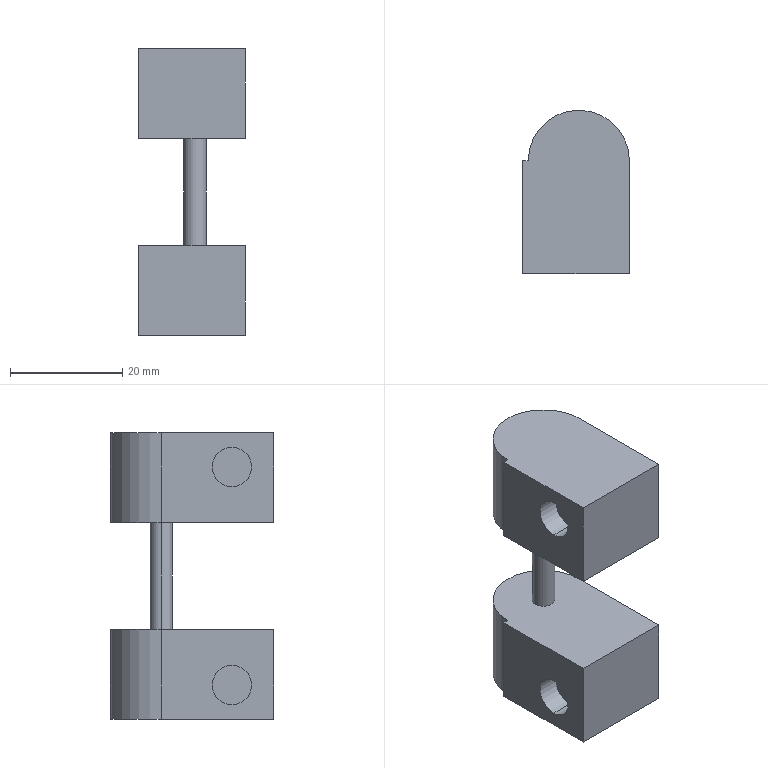Part | STEP file | Hinge side | 1 solid | 22 faces | box 19 x 29 x 51 mm | volume 16162 mm3 | plane 14 | cylinder 8 | commonest cylinder face diameters 7 x4 4 x2 18 x2
STEP:
#1=CARTESIAN_POINT('',(0.,0.,0.));
#2=DIRECTION('',(0.,0.,1.));
#3=DIRECTION('',(1.,0.,0.));
#4=AXIS2_PLACEMENT_3D('',#1,#2,#3);
#5=CARTESIAN_POINT('',(-6.,7.4,5.4));
#6=VERTEX_POINT('',#5);
#7=CARTESIAN_POINT('',(-10.,7.4,5.4));
#8=VERTEX_POINT('',#7);
#9=CARTESIAN_POINT('',(-6.,7.4,5.4));
#10=DIRECTION('',(-1.,0.,0.));
#11=VECTOR('',#10,1.);
#12=LINE('',#9,#11);
#13=CARTESIAN_POINT('',(-6.,7.4,1.9));
#14=DIRECTION('',(-1.,0.,0.));
#15=DIRECTION('',(0.,0.,1.));
#16=AXIS2_PLACEMENT_3D('',#13,#14,#15);
#17=CYLINDRICAL_SURFACE('',#16,3.5);
#18=CARTESIAN_POINT('',(6.283,0.));
#19=DIRECTION('',(0.,1.));
#20=VECTOR('',#19,1.);
#21=LINE('',#18,#20);
#22=(GEOMETRIC_REPRESENTATION_CONTEXT(2)PARAMETRIC_REPRESENTATION_CONTEXT()REPRESENTATION_CONTEXT('',''));
#23=DEFINITIONAL_REPRESENTATION('',(#21),#22);
#24=PCURVE('',#17,#23);
#25=CARTESIAN_POINT('',(-6.,7.4,1.9));
#26=DIRECTION('',(-1.,0.,0.));
#27=DIRECTION('',(0.,0.,1.));
#28=AXIS2_PLACEMENT_3D('',#25,#26,#27);
#29=CYLINDRICAL_SURFACE('',#28,3.5);
#30=CARTESIAN_POINT('',(0.,0.));
#31=DIRECTION('',(0.,1.));
#32=VECTOR('',#31,1.);
#33=LINE('',#30,#32);
#34=(GEOMETRIC_REPRESENTATION_CONTEXT(2)PARAMETRIC_REPRESENTATION_CONTEXT()REPRESENTATION_CONTEXT('',''));
#35=DEFINITIONAL_REPRESENTATION('',(#33),#34);
#36=PCURVE('',#29,#35);
#37=SURFACE_CURVE('',#12,(#24,#36),.PCURVE_S1.);
#38=EDGE_CURVE('',#6,#8,#37,.T.);
#39=ORIENTED_EDGE('',*,*,#38,.T.);
#40=CARTESIAN_POINT('',(-10.,7.4,-1.6));
#41=VERTEX_POINT('',#40);
#42=CARTESIAN_POINT('',(-10.,7.4,1.9));
#43=DIRECTION('',(-1.,0.,0.));
#44=DIRECTION('',(0.,0.,-1.));
#45=AXIS2_PLACEMENT_3D('',#42,#43,#44);
#46=CIRCLE('',#45,3.5);
#47=CARTESIAN_POINT('',(3.142,4.));
#48=DIRECTION('',(1.,0.));
#49=VECTOR('',#48,1.);
#50=LINE('',#47,#49);
#51=(GEOMETRIC_REPRESENTATION_CONTEXT(2)PARAMETRIC_REPRESENTATION_CONTEXT()REPRESENTATION_CONTEXT('',''));
#52=DEFINITIONAL_REPRESENTATION('',(#50),#51);
#53=PCURVE('',#17,#52);
#54=CARTESIAN_POINT('',(-10.,20.,8.));
#55=DIRECTION('',(-1.,0.,0.));
#56=DIRECTION('',(0.,0.,1.));
#57=AXIS2_PLACEMENT_3D('',#54,#55,#56);
#58=PLANE('',#57);
#59=CARTESIAN_POINT('',(-6.1,-12.6));
#60=DIRECTION('',(-1.,0.));
#61=AXIS2_PLACEMENT_2D('',#59,#60);
#62=CIRCLE('',#61,3.5);
#63=(GEOMETRIC_REPRESENTATION_CONTEXT(2)PARAMETRIC_REPRESENTATION_CONTEXT()REPRESENTATION_CONTEXT('',''));
#64=DEFINITIONAL_REPRESENTATION('',(#62),#63);
#65=PCURVE('',#58,#64);
#66=SURFACE_CURVE('',#46,(#53,#65),.PCURVE_S1.);
#67=EDGE_CURVE('',#41,#8,#66,.T.);
#68=ORIENTED_EDGE('',*,*,#67,.F.);
#69=CARTESIAN_POINT('',(-6.,7.4,-1.6));
#70=VERTEX_POINT('',#69);
#71=CARTESIAN_POINT('',(-6.,7.4,-1.6));
#72=DIRECTION('',(-1.,0.,0.));
#73=VECTOR('',#72,1.);
#74=LINE('',#71,#73);
#75=CARTESIAN_POINT('',(3.142,0.));
#76=DIRECTION('',(0.,1.));
#77=VECTOR('',#76,1.);
#78=LINE('',#75,#77);
#79=(GEOMETRIC_REPRESENTATION_CONTEXT(2)PARAMETRIC_REPRESENTATION_CONTEXT()REPRESENTATION_CONTEXT('',''));
#80=DEFINITIONAL_REPRESENTATION('',(#78),#79);
#81=PCURVE('',#17,#80);
#82=CARTESIAN_POINT('',(3.142,0.));
#83=DIRECTION('',(0.,1.));
#84=VECTOR('',#83,1.);
#85=LINE('',#82,#84);
#86=(GEOMETRIC_REPRESENTATION_CONTEXT(2)PARAMETRIC_REPRESENTATION_CONTEXT()REPRESENTATION_CONTEXT('',''));
#87=DEFINITIONAL_REPRESENTATION('',(#85),#86);
#88=PCURVE('',#29,#87);
#89=SURFACE_CURVE('',#74,(#81,#88),.PCURVE_S1.);
#90=EDGE_CURVE('',#70,#41,#89,.T.);
#91=ORIENTED_EDGE('',*,*,#90,.F.);
#92=CARTESIAN_POINT('',(-6.,7.4,1.9));
#93=DIRECTION('',(-1.,0.,0.));
#94=DIRECTION('',(0.,0.,-1.));
#95=AXIS2_PLACEMENT_3D('',#92,#93,#94);
#96=CIRCLE('',#95,3.5);
#97=CARTESIAN_POINT('',(3.142,0.));
#98=DIRECTION('',(1.,0.));
#99=VECTOR('',#98,1.);
#100=LINE('',#97,#99);
#101=(GEOMETRIC_REPRESENTATION_CONTEXT(2)PARAMETRIC_REPRESENTATION_CONTEXT()REPRESENTATION_CONTEXT('',''));
#102=DEFINITIONAL_REPRESENTATION('',(#100),#101);
#103=PCURVE('',#17,#102);
#104=CARTESIAN_POINT('',(-6.,7.4,1.9));
#105=DIRECTION('',(1.,0.,0.));
#106=DIRECTION('',(0.,0.,-1.));
#107=AXIS2_PLACEMENT_3D('',#104,#105,#106);
#108=PLANE('',#107);
#109=CARTESIAN_POINT('',(3.5,0.));
#110=CARTESIAN_POINT('',(3.5,-6.062));
#111=CARTESIAN_POINT('',(-1.75,-3.031));
#112=CARTESIAN_POINT('',(-7.,0.));
#113=CARTESIAN_POINT('',(-1.75,3.031));
#114=CARTESIAN_POINT('',(3.5,6.062));
#115=CARTESIAN_POINT('',(3.5,0.));
#116=(BOUNDED_CURVE()B_SPLINE_CURVE(2,(#109,#110,#111,#112,#113,#114,#115),.UNSPECIFIED.,.T.,.F.)B_SPLINE_CURVE_WITH_KNOTS((1,2,2,2,2,1),(-2.094,0.,2.094,4.189,6.283,8.378),.UNSPECIFIED.)CURVE()GEOMETRIC_REPRESENTATION_ITEM()RATIONAL_B_SPLINE_CURVE((1.,0.5,1.,0.5,1.,0.5,1.))REPRESENTATION_ITEM(''));
#117=(GEOMETRIC_REPRESENTATION_CONTEXT(2)PARAMETRIC_REPRESENTATION_CONTEXT()REPRESENTATION_CONTEXT('',''));
#118=DEFINITIONAL_REPRESENTATION('',(#116),#117);
#119=PCURVE('',#108,#118);
#120=SURFACE_CURVE('',#96,(#103,#119),.PCURVE_S1.);
#121=EDGE_CURVE('',#70,#6,#120,.T.);
#122=ORIENTED_EDGE('',*,*,#121,.T.);
#123=EDGE_LOOP('',(#39,#68,#91,#122));
#124=FACE_BOUND('',#123,.F.);
#125=ADVANCED_FACE('',(#124),#17,.F.);
#126=CARTESIAN_POINT('',(-6.,7.4,-33.4));
#127=VERTEX_POINT('',#126);
#128=CARTESIAN_POINT('',(-10.,7.4,-33.4));
#129=VERTEX_POINT('',#128);
#130=CARTESIAN_POINT('',(-6.,7.4,-33.4));
#131=DIRECTION('',(-1.,0.,0.));
#132=VECTOR('',#131,1.);
#133=LINE('',#130,#132);
#134=CARTESIAN_POINT('',(-6.,7.4,-36.9));
#135=DIRECTION('',(-1.,0.,0.));
#136=DIRECTION('',(0.,0.,1.));
#137=AXIS2_PLACEMENT_3D('',#134,#135,#136);
#138=CYLINDRICAL_SURFACE('',#137,3.5);
#139=CARTESIAN_POINT('',(6.283,0.));
#140=DIRECTION('',(0.,1.));
#141=VECTOR('',#140,1.);
#142=LINE('',#139,#141);
#143=(GEOMETRIC_REPRESENTATION_CONTEXT(2)PARAMETRIC_REPRESENTATION_CONTEXT()REPRESENTATION_CONTEXT('',''));
#144=DEFINITIONAL_REPRESENTATION('',(#142),#143);
#145=PCURVE('',#138,#144);
#146=CARTESIAN_POINT('',(-6.,7.4,-36.9));
#147=DIRECTION('',(-1.,0.,0.));
#148=DIRECTION('',(0.,0.,1.));
#149=AXIS2_PLACEMENT_3D('',#146,#147,#148);
#150=CYLINDRICAL_SURFACE('',#149,3.5);
#151=CARTESIAN_POINT('',(0.,0.));
#152=DIRECTION('',(0.,1.));
#153=VECTOR('',#152,1.);
#154=LINE('',#151,#153);
#155=(GEOMETRIC_REPRESENTATION_CONTEXT(2)PARAMETRIC_REPRESENTATION_CONTEXT()REPRESENTATION_CONTEXT('',''));
#156=DEFINITIONAL_REPRESENTATION('',(#154),#155);
#157=PCURVE('',#150,#156);
#158=SURFACE_CURVE('',#133,(#145,#157),.PCURVE_S1.);
#159=EDGE_CURVE('',#127,#129,#158,.T.);
#160=ORIENTED_EDGE('',*,*,#159,.T.);
#161=CARTESIAN_POINT('',(-10.,7.4,-40.4));
#162=VERTEX_POINT('',#161);
#163=CARTESIAN_POINT('',(-10.,7.4,-36.9));
#164=DIRECTION('',(-1.,0.,0.));
#165=DIRECTION('',(0.,0.,1.));
#166=AXIS2_PLACEMENT_3D('',#163,#164,#165);
#167=CIRCLE('',#166,3.5);
#168=CARTESIAN_POINT('',(0.,4.));
#169=DIRECTION('',(1.,0.));
#170=VECTOR('',#169,1.);
#171=LINE('',#168,#170);
#172=(GEOMETRIC_REPRESENTATION_CONTEXT(2)PARAMETRIC_REPRESENTATION_CONTEXT()REPRESENTATION_CONTEXT('',''));
#173=DEFINITIONAL_REPRESENTATION('',(#171),#172);
#174=PCURVE('',#138,#173);
#175=CARTESIAN_POINT('',(-10.,20.,-43.));
#176=DIRECTION('',(1.,0.,0.));
#177=DIRECTION('',(0.,0.,-1.));
#178=AXIS2_PLACEMENT_3D('',#175,#176,#177);
#179=PLANE('',#178);
#180=CARTESIAN_POINT('',(-9.6,-12.6));
#181=CARTESIAN_POINT('',(-9.6,-6.538));
#182=CARTESIAN_POINT('',(-4.35,-9.569));
#183=CARTESIAN_POINT('',(0.9,-12.6));
#184=CARTESIAN_POINT('',(-4.35,-15.631));
#185=CARTESIAN_POINT('',(-9.6,-18.662));
#186=CARTESIAN_POINT('',(-9.6,-12.6));
#187=(BOUNDED_CURVE()B_SPLINE_CURVE(2,(#180,#181,#182,#183,#184,#185,#186),.UNSPECIFIED.,.T.,.F.)B_SPLINE_CURVE_WITH_KNOTS((1,2,2,2,2,1),(-2.094,0.,2.094,4.189,6.283,8.378),.UNSPECIFIED.)CURVE()GEOMETRIC_REPRESENTATION_ITEM()RATIONAL_B_SPLINE_CURVE((1.,0.5,1.,0.5,1.,0.5,1.))REPRESENTATION_ITEM(''));
#188=(GEOMETRIC_REPRESENTATION_CONTEXT(2)PARAMETRIC_REPRESENTATION_CONTEXT()REPRESENTATION_CONTEXT('',''));
#189=DEFINITIONAL_REPRESENTATION('',(#187),#188);
#190=PCURVE('',#179,#189);
#191=SURFACE_CURVE('',#167,(#174,#190),.PCURVE_S1.);
#192=EDGE_CURVE('',#162,#129,#191,.T.);
#193=ORIENTED_EDGE('',*,*,#192,.F.);
#194=CARTESIAN_POINT('',(-6.,7.4,-40.4));
#195=VERTEX_POINT('',#194);
#196=CARTESIAN_POINT('',(-6.,7.4,-40.4));
#197=DIRECTION('',(-1.,0.,0.));
#198=VECTOR('',#197,1.);
#199=LINE('',#196,#198);
#200=CARTESIAN_POINT('',(3.142,0.));
#201=DIRECTION('',(0.,1.));
#202=VECTOR('',#201,1.);
#203=LINE('',#200,#202);
#204=(GEOMETRIC_REPRESENTATION_CONTEXT(2)PARAMETRIC_REPRESENTATION_CONTEXT()REPRESENTATION_CONTEXT('',''));
#205=DEFINITIONAL_REPRESENTATION('',(#203),#204);
#206=PCURVE('',#138,#205);
#207=CARTESIAN_POINT('',(3.142,0.));
#208=DIRECTION('',(0.,1.));
#209=VECTOR('',#208,1.);
#210=LINE('',#207,#209);
#211=(GEOMETRIC_REPRESENTATION_CONTEXT(2)PARAMETRIC_REPRESENTATION_CONTEXT()REPRESENTATION_CONTEXT('',''));
#212=DEFINITIONAL_REPRESENTATION('',(#210),#211);
#213=PCURVE('',#150,#212);
#214=SURFACE_CURVE('',#199,(#206,#213),.PCURVE_S1.);
#215=EDGE_CURVE('',#195,#162,#214,.T.);
#216=ORIENTED_EDGE('',*,*,#215,.F.);
#217=CARTESIAN_POINT('',(-6.,7.4,-36.9));
#218=DIRECTION('',(-1.,0.,0.));
#219=DIRECTION('',(0.,0.,1.));
#220=AXIS2_PLACEMENT_3D('',#217,#218,#219);
#221=CIRCLE('',#220,3.5);
#222=CARTESIAN_POINT('',(0.,0.));
#223=DIRECTION('',(1.,0.));
#224=VECTOR('',#223,1.);
#225=LINE('',#222,#224);
#226=(GEOMETRIC_REPRESENTATION_CONTEXT(2)PARAMETRIC_REPRESENTATION_CONTEXT()REPRESENTATION_CONTEXT('',''));
#227=DEFINITIONAL_REPRESENTATION('',(#225),#226);
#228=PCURVE('',#138,#227);
#229=CARTESIAN_POINT('',(-6.,7.4,-36.9));
#230=DIRECTION('',(-1.,0.,0.));
#231=DIRECTION('',(0.,0.,1.));
#232=AXIS2_PLACEMENT_3D('',#229,#230,#231);
#233=PLANE('',#232);
#234=CARTESIAN_POINT('',(0.,0.));
#235=DIRECTION('',(1.,0.));
#236=AXIS2_PLACEMENT_2D('',#234,#235);
#237=CIRCLE('',#236,3.5);
#238=(GEOMETRIC_REPRESENTATION_CONTEXT(2)PARAMETRIC_REPRESENTATION_CONTEXT()REPRESENTATION_CONTEXT('',''));
#239=DEFINITIONAL_REPRESENTATION('',(#237),#238);
#240=PCURVE('',#233,#239);
#241=SURFACE_CURVE('',#221,(#228,#240),.PCURVE_S1.);
#242=EDGE_CURVE('',#195,#127,#241,.T.);
#243=ORIENTED_EDGE('',*,*,#242,.T.);
#244=EDGE_LOOP('',(#160,#193,#216,#243));
#245=FACE_BOUND('',#244,.F.);
#246=ADVANCED_FACE('',(#245),#138,.F.);
#247=CARTESIAN_POINT('',(-2.,20.,-27.));
#248=VERTEX_POINT('',#247);
#249=CARTESIAN_POINT('',(2.,20.,-27.));
#250=VERTEX_POINT('',#249);
#251=CARTESIAN_POINT('',(0.,20.,-27.));
#252=DIRECTION('',(0.,0.,-1.));
#253=DIRECTION('',(-1.,0.,0.));
#254=AXIS2_PLACEMENT_3D('',#251,#252,#253);
#255=CIRCLE('',#254,2.);
#256=CARTESIAN_POINT('',(0.,20.,-27.));
#257=DIRECTION('',(0.,0.,1.));
#258=DIRECTION('',(1.,0.,0.));
#259=AXIS2_PLACEMENT_3D('',#256,#257,#258);
#260=CYLINDRICAL_SURFACE('',#259,2.);
#261=CARTESIAN_POINT('',(3.142,0.));
#262=DIRECTION('',(-1.,0.));
#263=VECTOR('',#262,1.);
#264=LINE('',#261,#263);
#265=(GEOMETRIC_REPRESENTATION_CONTEXT(2)PARAMETRIC_REPRESENTATION_CONTEXT()REPRESENTATION_CONTEXT('',''));
#266=DEFINITIONAL_REPRESENTATION('',(#264),#265);
#267=PCURVE('',#260,#266);
#268=CARTESIAN_POINT('',(-9.,20.,-27.));
#269=DIRECTION('',(0.,0.,1.));
#270=DIRECTION('',(1.,0.,0.));
#271=AXIS2_PLACEMENT_3D('',#268,#269,#270);
#272=PLANE('',#271);
#273=CARTESIAN_POINT('',(7.,0.));
#274=CARTESIAN_POINT('',(7.,3.464));
#275=CARTESIAN_POINT('',(10.,1.732));
#276=CARTESIAN_POINT('',(13.,0.));
#277=CARTESIAN_POINT('',(10.,-1.732));
#278=CARTESIAN_POINT('',(7.,-3.464));
#279=CARTESIAN_POINT('',(7.,0.));
#280=(BOUNDED_CURVE()B_SPLINE_CURVE(2,(#273,#274,#275,#276,#277,#278,#279),.UNSPECIFIED.,.T.,.F.)B_SPLINE_CURVE_WITH_KNOTS((1,2,2,2,2,1),(-2.094,0.,2.094,4.189,6.283,8.378),.UNSPECIFIED.)CURVE()GEOMETRIC_REPRESENTATION_ITEM()RATIONAL_B_SPLINE_CURVE((1.,0.5,1.,0.5,1.,0.5,1.))REPRESENTATION_ITEM(''));
#281=(GEOMETRIC_REPRESENTATION_CONTEXT(2)PARAMETRIC_REPRESENTATION_CONTEXT()REPRESENTATION_CONTEXT('',''));
#282=DEFINITIONAL_REPRESENTATION('',(#280),#281);
#283=PCURVE('',#272,#282);
#284=SURFACE_CURVE('',#255,(#267,#283),.PCURVE_S1.);
#285=EDGE_CURVE('',#248,#250,#284,.T.);
#286=ORIENTED_EDGE('',*,*,#285,.F.);
#287=CARTESIAN_POINT('',(-2.,20.,-8.));
#288=VERTEX_POINT('',#287);
#289=CARTESIAN_POINT('',(-2.,20.,-27.));
#290=DIRECTION('',(0.,0.,1.));
#291=VECTOR('',#290,1.);
#292=LINE('',#289,#291);
#293=CARTESIAN_POINT('',(3.142,0.));
#294=DIRECTION('',(0.,1.));
#295=VECTOR('',#294,1.);
#296=LINE('',#293,#295);
#297=(GEOMETRIC_REPRESENTATION_CONTEXT(2)PARAMETRIC_REPRESENTATION_CONTEXT()REPRESENTATION_CONTEXT('',''));
#298=DEFINITIONAL_REPRESENTATION('',(#296),#297);
#299=PCURVE('',#260,#298);
#300=CARTESIAN_POINT('',(0.,20.,-27.));
#301=DIRECTION('',(0.,0.,1.));
#302=DIRECTION('',(1.,0.,0.));
#303=AXIS2_PLACEMENT_3D('',#300,#301,#302);
#304=CYLINDRICAL_SURFACE('',#303,2.);
#305=CARTESIAN_POINT('',(3.142,0.));
#306=DIRECTION('',(0.,1.));
#307=VECTOR('',#306,1.);
#308=LINE('',#305,#307);
#309=(GEOMETRIC_REPRESENTATION_CONTEXT(2)PARAMETRIC_REPRESENTATION_CONTEXT()REPRESENTATION_CONTEXT('',''));
#310=DEFINITIONAL_REPRESENTATION('',(#308),#309);
#311=PCURVE('',#304,#310);
#312=SURFACE_CURVE('',#292,(#299,#311),.PCURVE_S1.);
#313=EDGE_CURVE('',#248,#288,#312,.T.);
#314=ORIENTED_EDGE('',*,*,#313,.T.);
#315=CARTESIAN_POINT('',(2.,20.,-8.));
#316=VERTEX_POINT('',#315);
#317=CARTESIAN_POINT('',(0.,20.,-8.));
#318=DIRECTION('',(0.,0.,-1.));
#319=DIRECTION('',(1.,0.,0.));
#320=AXIS2_PLACEMENT_3D('',#317,#318,#319);
#321=CIRCLE('',#320,2.);
#322=CARTESIAN_POINT('',(6.283,19.));
#323=DIRECTION('',(-1.,0.));
#324=VECTOR('',#323,1.);
#325=LINE('',#322,#324);
#326=(GEOMETRIC_REPRESENTATION_CONTEXT(2)PARAMETRIC_REPRESENTATION_CONTEXT()REPRESENTATION_CONTEXT('',''));
#327=DEFINITIONAL_REPRESENTATION('',(#325),#326);
#328=PCURVE('',#260,#327);
#329=CARTESIAN_POINT('',(-9.,20.,-8.));
#330=DIRECTION('',(0.,0.,1.));
#331=DIRECTION('',(1.,0.,0.));
#332=AXIS2_PLACEMENT_3D('',#329,#330,#331);
#333=PLANE('',#332);
#334=CARTESIAN_POINT('',(11.,0.));
#335=CARTESIAN_POINT('',(11.,-3.464));
#336=CARTESIAN_POINT('',(8.,-1.732));
#337=CARTESIAN_POINT('',(5.,0.));
#338=CARTESIAN_POINT('',(8.,1.732));
#339=CARTESIAN_POINT('',(11.,3.464));
#340=CARTESIAN_POINT('',(11.,0.));
#341=(BOUNDED_CURVE()B_SPLINE_CURVE(2,(#334,#335,#336,#337,#338,#339,#340),.UNSPECIFIED.,.T.,.F.)B_SPLINE_CURVE_WITH_KNOTS((1,2,2,2,2,1),(-2.094,0.,2.094,4.189,6.283,8.378),.UNSPECIFIED.)CURVE()GEOMETRIC_REPRESENTATION_ITEM()RATIONAL_B_SPLINE_CURVE((1.,0.5,1.,0.5,1.,0.5,1.))REPRESENTATION_ITEM(''));
#342=(GEOMETRIC_REPRESENTATION_CONTEXT(2)PARAMETRIC_REPRESENTATION_CONTEXT()REPRESENTATION_CONTEXT('',''));
#343=DEFINITIONAL_REPRESENTATION('',(#341),#342);
#344=PCURVE('',#333,#343);
#345=SURFACE_CURVE('',#321,(#328,#344),.PCURVE_S1.);
#346=EDGE_CURVE('',#288,#316,#345,.T.);
#347=ORIENTED_EDGE('',*,*,#346,.T.);
#348=CARTESIAN_POINT('',(2.,20.,-27.));
#349=DIRECTION('',(0.,0.,1.));
#350=VECTOR('',#349,1.);
#351=LINE('',#348,#350);
#352=CARTESIAN_POINT('',(0.,0.));
#353=DIRECTION('',(0.,1.));
#354=VECTOR('',#353,1.);
#355=LINE('',#352,#354);
#356=(GEOMETRIC_REPRESENTATION_CONTEXT(2)PARAMETRIC_REPRESENTATION_CONTEXT()REPRESENTATION_CONTEXT('',''));
#357=DEFINITIONAL_REPRESENTATION('',(#355),#356);
#358=PCURVE('',#260,#357);
#359=CARTESIAN_POINT('',(6.283,0.));
#360=DIRECTION('',(0.,1.));
#361=VECTOR('',#360,1.);
#362=LINE('',#359,#361);
#363=(GEOMETRIC_REPRESENTATION_CONTEXT(2)PARAMETRIC_REPRESENTATION_CONTEXT()REPRESENTATION_CONTEXT('',''));
#364=DEFINITIONAL_REPRESENTATION('',(#362),#363);
#365=PCURVE('',#304,#364);
#366=SURFACE_CURVE('',#351,(#358,#365),.PCURVE_S1.);
#367=EDGE_CURVE('',#250,#316,#366,.T.);
#368=ORIENTED_EDGE('',*,*,#367,.F.);
#369=EDGE_LOOP('',(#286,#314,#347,#368));
#370=FACE_BOUND('',#369,.T.);
#371=ADVANCED_FACE('',(#370),#260,.T.);
#372=CARTESIAN_POINT('',(9.,0.,8.));
#373=VERTEX_POINT('',#372);
#374=CARTESIAN_POINT('',(9.,0.,-8.));
#375=VERTEX_POINT('',#374);
#376=CARTESIAN_POINT('',(9.,0.,-8.));
#377=DIRECTION('',(0.,0.,-1.));
#378=VECTOR('',#377,1.);
#379=LINE('',#376,#378);
#380=CARTESIAN_POINT('',(9.,20.,-8.));
#381=DIRECTION('',(-1.,0.,0.));
#382=DIRECTION('',(0.,0.,1.));
#383=AXIS2_PLACEMENT_3D('',#380,#381,#382);
#384=PLANE('',#383);
#385=CARTESIAN_POINT('',(0.,-20.));
#386=DIRECTION('',(-1.,0.));
#387=VECTOR('',#386,1.);
#388=LINE('',#385,#387);
#389=(GEOMETRIC_REPRESENTATION_CONTEXT(2)PARAMETRIC_REPRESENTATION_CONTEXT()REPRESENTATION_CONTEXT('',''));
#390=DEFINITIONAL_REPRESENTATION('',(#388),#389);
#391=PCURVE('',#384,#390);
#392=CARTESIAN_POINT('',(0.,0.,0.));
#393=DIRECTION('',(0.,1.,0.));
#394=DIRECTION('',(0.,0.,1.));
#395=AXIS2_PLACEMENT_3D('',#392,#393,#394);
#396=PLANE('',#395);
#397=CARTESIAN_POINT('',(-8.,9.));
#398=DIRECTION('',(-1.,0.));
#399=VECTOR('',#398,1.);
#400=LINE('',#397,#399);
#401=(GEOMETRIC_REPRESENTATION_CONTEXT(2)PARAMETRIC_REPRESENTATION_CONTEXT()REPRESENTATION_CONTEXT('',''));
#402=DEFINITIONAL_REPRESENTATION('',(#400),#401);
#403=PCURVE('',#396,#402);
#404=SURFACE_CURVE('',#379,(#391,#403),.PCURVE_S1.);
#405=EDGE_CURVE('',#373,#375,#404,.T.);
#406=ORIENTED_EDGE('',*,*,#405,.T.);
#407=CARTESIAN_POINT('',(9.,20.,-8.));
#408=VERTEX_POINT('',#407);
#409=CARTESIAN_POINT('',(9.,20.,-8.));
#410=DIRECTION('',(0.,-1.,0.));
#411=VECTOR('',#410,1.);
#412=LINE('',#409,#411);
#413=CARTESIAN_POINT('',(0.,0.));
#414=DIRECTION('',(0.,-1.));
#415=VECTOR('',#414,1.);
#416=LINE('',#413,#415);
#417=(GEOMETRIC_REPRESENTATION_CONTEXT(2)PARAMETRIC_REPRESENTATION_CONTEXT()REPRESENTATION_CONTEXT('',''));
#418=DEFINITIONAL_REPRESENTATION('',(#416),#417);
#419=PCURVE('',#384,#418);
#420=CARTESIAN_POINT('',(18.,0.));
#421=DIRECTION('',(0.,-1.));
#422=VECTOR('',#421,1.);
#423=LINE('',#420,#422);
#424=(GEOMETRIC_REPRESENTATION_CONTEXT(2)PARAMETRIC_REPRESENTATION_CONTEXT()REPRESENTATION_CONTEXT('',''));
#425=DEFINITIONAL_REPRESENTATION('',(#423),#424);
#426=PCURVE('',#333,#425);
#427=SURFACE_CURVE('',#412,(#419,#426),.PCURVE_S1.);
#428=EDGE_CURVE('',#408,#375,#427,.T.);
#429=ORIENTED_EDGE('',*,*,#428,.F.);
#430=CARTESIAN_POINT('',(9.,20.,8.));
#431=VERTEX_POINT('',#430);
#432=CARTESIAN_POINT('',(9.,20.,-8.));
#433=DIRECTION('',(0.,0.,-1.));
#434=VECTOR('',#433,1.);
#435=LINE('',#432,#434);
#436=CARTESIAN_POINT('',(0.,0.));
#437=DIRECTION('',(-1.,0.));
#438=VECTOR('',#437,1.);
#439=LINE('',#436,#438);
#440=(GEOMETRIC_REPRESENTATION_CONTEXT(2)PARAMETRIC_REPRESENTATION_CONTEXT()REPRESENTATION_CONTEXT('',''));
#441=DEFINITIONAL_REPRESENTATION('',(#439),#440);
#442=PCURVE('',#384,#441);
#443=CARTESIAN_POINT('',(0.,20.,8.));
#444=DIRECTION('',(0.,0.,-1.));
#445=DIRECTION('',(-1.,0.,0.));
#446=AXIS2_PLACEMENT_3D('',#443,#444,#445);
#447=CYLINDRICAL_SURFACE('',#446,9.);
#448=CARTESIAN_POINT('',(3.142,16.));
#449=DIRECTION('',(0.,1.));
#450=VECTOR('',#449,1.);
#451=LINE('',#448,#450);
#452=(GEOMETRIC_REPRESENTATION_CONTEXT(2)PARAMETRIC_REPRESENTATION_CONTEXT()REPRESENTATION_CONTEXT('',''));
#453=DEFINITIONAL_REPRESENTATION('',(#451),#452);
#454=PCURVE('',#447,#453);
#455=SURFACE_CURVE('',#435,(#442,#454),.PCURVE_S1.);
#456=EDGE_CURVE('',#431,#408,#455,.T.);
#457=ORIENTED_EDGE('',*,*,#456,.F.);
#458=CARTESIAN_POINT('',(9.,20.,8.));
#459=DIRECTION('',(0.,-1.,0.));
#460=VECTOR('',#459,1.);
#461=LINE('',#458,#460);
#462=CARTESIAN_POINT('',(16.,0.));
#463=DIRECTION('',(0.,-1.));
#464=VECTOR('',#463,1.);
#465=LINE('',#462,#464);
#466=(GEOMETRIC_REPRESENTATION_CONTEXT(2)PARAMETRIC_REPRESENTATION_CONTEXT()REPRESENTATION_CONTEXT('',''));
#467=DEFINITIONAL_REPRESENTATION('',(#465),#466);
#468=PCURVE('',#384,#467);
#469=CARTESIAN_POINT('',(-9.,20.,8.));
#470=DIRECTION('',(0.,0.,-1.));
#471=DIRECTION('',(-1.,0.,0.));
#472=AXIS2_PLACEMENT_3D('',#469,#470,#471);
#473=PLANE('',#472);
#474=CARTESIAN_POINT('',(-18.,0.));
#475=DIRECTION('',(0.,-1.));
#476=VECTOR('',#475,1.);
#477=LINE('',#474,#476);
#478=(GEOMETRIC_REPRESENTATION_CONTEXT(2)PARAMETRIC_REPRESENTATION_CONTEXT()REPRESENTATION_CONTEXT('',''));
#479=DEFINITIONAL_REPRESENTATION('',(#477),#478);
#480=PCURVE('',#473,#479);
#481=SURFACE_CURVE('',#461,(#468,#480),.PCURVE_S1.);
#482=EDGE_CURVE('',#431,#373,#481,.T.);
#483=ORIENTED_EDGE('',*,*,#482,.T.);
#484=EDGE_LOOP('',(#406,#429,#457,#483));
#485=FACE_BOUND('',#484,.T.);
#486=ADVANCED_FACE('',(#485),#384,.F.);
#487=CARTESIAN_POINT('',(0.,20.,-8.));
#488=DIRECTION('',(0.,0.,-1.));
#489=DIRECTION('',(1.,0.,0.));
#490=AXIS2_PLACEMENT_3D('',#487,#488,#489);
#491=CIRCLE('',#490,2.);
#492=CARTESIAN_POINT('',(11.,0.));
#493=CARTESIAN_POINT('',(11.,-3.464));
#494=CARTESIAN_POINT('',(8.,-1.732));
#495=CARTESIAN_POINT('',(5.,0.));
#496=CARTESIAN_POINT('',(8.,1.732));
#497=CARTESIAN_POINT('',(11.,3.464));
#498=CARTESIAN_POINT('',(11.,0.));
#499=(BOUNDED_CURVE()B_SPLINE_CURVE(2,(#492,#493,#494,#495,#496,#497,#498),.UNSPECIFIED.,.T.,.F.)B_SPLINE_CURVE_WITH_KNOTS((1,2,2,2,2,1),(-2.094,0.,2.094,4.189,6.283,8.378),.UNSPECIFIED.)CURVE()GEOMETRIC_REPRESENTATION_ITEM()RATIONAL_B_SPLINE_CURVE((1.,0.5,1.,0.5,1.,0.5,1.))REPRESENTATION_ITEM(''));
#500=(GEOMETRIC_REPRESENTATION_CONTEXT(2)PARAMETRIC_REPRESENTATION_CONTEXT()REPRESENTATION_CONTEXT('',''));
#501=DEFINITIONAL_REPRESENTATION('',(#499),#500);
#502=PCURVE('',#333,#501);
#503=CARTESIAN_POINT('',(6.283,19.));
#504=DIRECTION('',(-1.,0.));
#505=VECTOR('',#504,1.);
#506=LINE('',#503,#505);
#507=(GEOMETRIC_REPRESENTATION_CONTEXT(2)PARAMETRIC_REPRESENTATION_CONTEXT()REPRESENTATION_CONTEXT('',''));
#508=DEFINITIONAL_REPRESENTATION('',(#506),#507);
#509=PCURVE('',#304,#508);
#510=SURFACE_CURVE('',#491,(#502,#509),.PCURVE_S1.);
#511=EDGE_CURVE('',#316,#288,#510,.T.);
#512=ORIENTED_EDGE('',*,*,#511,.F.);
#513=ORIENTED_EDGE('',*,*,#346,.F.);
#514=EDGE_LOOP('',(#512,#513));
#515=FACE_BOUND('',#514,.T.);
#516=CARTESIAN_POINT('',(-10.,0.,-8.));
#517=VERTEX_POINT('',#516);
#518=CARTESIAN_POINT('',(-9.,0.,-8.));
#519=DIRECTION('',(-1.,0.,0.));
#520=VECTOR('',#519,1.);
#521=LINE('',#518,#520);
#522=CARTESIAN_POINT('',(0.,-20.));
#523=DIRECTION('',(-1.,0.));
#524=VECTOR('',#523,1.);
#525=LINE('',#522,#524);
#526=(GEOMETRIC_REPRESENTATION_CONTEXT(2)PARAMETRIC_REPRESENTATION_CONTEXT()REPRESENTATION_CONTEXT('',''));
#527=DEFINITIONAL_REPRESENTATION('',(#525),#526);
#528=PCURVE('',#333,#527);
#529=CARTESIAN_POINT('',(-8.,-9.));
#530=DIRECTION('',(0.,-1.));
#531=VECTOR('',#530,1.);
#532=LINE('',#529,#531);
#533=(GEOMETRIC_REPRESENTATION_CONTEXT(2)PARAMETRIC_REPRESENTATION_CONTEXT()REPRESENTATION_CONTEXT('',''));
#534=DEFINITIONAL_REPRESENTATION('',(#532),#533);
#535=PCURVE('',#396,#534);
#536=SURFACE_CURVE('',#521,(#528,#535),.PCURVE_S1.);
#537=EDGE_CURVE('',#375,#517,#536,.T.);
#538=ORIENTED_EDGE('',*,*,#537,.T.);
#539=CARTESIAN_POINT('',(-10.,20.,-8.));
#540=VERTEX_POINT('',#539);
#541=CARTESIAN_POINT('',(-10.,20.,-8.));
#542=DIRECTION('',(0.,-1.,0.));
#543=VECTOR('',#542,1.);
#544=LINE('',#541,#543);
#545=CARTESIAN_POINT('',(-1.,0.));
#546=DIRECTION('',(0.,-1.));
#547=VECTOR('',#546,1.);
#548=LINE('',#545,#547);
#549=(GEOMETRIC_REPRESENTATION_CONTEXT(2)PARAMETRIC_REPRESENTATION_CONTEXT()REPRESENTATION_CONTEXT('',''));
#550=DEFINITIONAL_REPRESENTATION('',(#548),#549);
#551=PCURVE('',#333,#550);
#552=CARTESIAN_POINT('',(-16.,0.));
#553=DIRECTION('',(0.,-1.));
#554=VECTOR('',#553,1.);
#555=LINE('',#552,#554);
#556=(GEOMETRIC_REPRESENTATION_CONTEXT(2)PARAMETRIC_REPRESENTATION_CONTEXT()REPRESENTATION_CONTEXT('',''));
#557=DEFINITIONAL_REPRESENTATION('',(#555),#556);
#558=PCURVE('',#58,#557);
#559=SURFACE_CURVE('',#544,(#551,#558),.PCURVE_S1.);
#560=EDGE_CURVE('',#540,#517,#559,.T.);
#561=ORIENTED_EDGE('',*,*,#560,.F.);
#562=CARTESIAN_POINT('',(-9.,20.,-8.));
#563=VERTEX_POINT('',#562);
#564=CARTESIAN_POINT('',(-9.,20.,-8.));
#565=DIRECTION('',(1.,0.,0.));
#566=VECTOR('',#565,1.);
#567=LINE('',#564,#566);
#568=CARTESIAN_POINT('',(0.,0.));
#569=DIRECTION('',(1.,0.));
#570=VECTOR('',#569,1.);
#571=LINE('',#568,#570);
#572=(GEOMETRIC_REPRESENTATION_CONTEXT(2)PARAMETRIC_REPRESENTATION_CONTEXT()REPRESENTATION_CONTEXT('',''));
#573=DEFINITIONAL_REPRESENTATION('',(#571),#572);
#574=PCURVE('',#333,#573);
#575=CARTESIAN_POINT('',(0.,20.,0.));
#576=DIRECTION('',(0.,1.,0.));
#577=DIRECTION('',(0.,0.,1.));
#578=AXIS2_PLACEMENT_3D('',#575,#576,#577);
#579=PLANE('',#578);
#580=CARTESIAN_POINT('',(-8.,-9.));
#581=DIRECTION('',(0.,1.));
#582=VECTOR('',#581,1.);
#583=LINE('',#580,#582);
#584=(GEOMETRIC_REPRESENTATION_CONTEXT(2)PARAMETRIC_REPRESENTATION_CONTEXT()REPRESENTATION_CONTEXT('',''));
#585=DEFINITIONAL_REPRESENTATION('',(#583),#584);
#586=PCURVE('',#579,#585);
#587=SURFACE_CURVE('',#567,(#574,#586),.PCURVE_S1.);
#588=EDGE_CURVE('',#540,#563,#587,.T.);
#589=ORIENTED_EDGE('',*,*,#588,.T.);
#590=CARTESIAN_POINT('',(0.,20.,-8.));
#591=DIRECTION('',(0.,0.,-1.));
#592=DIRECTION('',(1.,0.,0.));
#593=AXIS2_PLACEMENT_3D('',#590,#591,#592);
#594=CIRCLE('',#593,9.);
#595=CARTESIAN_POINT('',(18.,0.));
#596=CARTESIAN_POINT('',(18.,-15.588));
#597=CARTESIAN_POINT('',(4.5,-7.794));
#598=CARTESIAN_POINT('',(-9.,0.));
#599=CARTESIAN_POINT('',(4.5,7.794));
#600=CARTESIAN_POINT('',(18.,15.588));
#601=CARTESIAN_POINT('',(18.,0.));
#602=(BOUNDED_CURVE()B_SPLINE_CURVE(2,(#595,#596,#597,#598,#599,#600,#601),.UNSPECIFIED.,.T.,.F.)B_SPLINE_CURVE_WITH_KNOTS((1,2,2,2,2,1),(-2.094,0.,2.094,4.189,6.283,8.378),.UNSPECIFIED.)CURVE()GEOMETRIC_REPRESENTATION_ITEM()RATIONAL_B_SPLINE_CURVE((1.,0.5,1.,0.5,1.,0.5,1.))REPRESENTATION_ITEM(''));
#603=(GEOMETRIC_REPRESENTATION_CONTEXT(2)PARAMETRIC_REPRESENTATION_CONTEXT()REPRESENTATION_CONTEXT('',''));
#604=DEFINITIONAL_REPRESENTATION('',(#602),#603);
#605=PCURVE('',#333,#604);
#606=CARTESIAN_POINT('',(-3.142,16.));
#607=DIRECTION('',(1.,0.));
#608=VECTOR('',#607,1.);
#609=LINE('',#606,#608);
#610=(GEOMETRIC_REPRESENTATION_CONTEXT(2)PARAMETRIC_REPRESENTATION_CONTEXT()REPRESENTATION_CONTEXT('',''));
#611=DEFINITIONAL_REPRESENTATION('',(#609),#610);
#612=PCURVE('',#447,#611);
#613=SURFACE_CURVE('',#594,(#605,#612),.PCURVE_S1.);
#614=EDGE_CURVE('',#563,#408,#613,.T.);
#615=ORIENTED_EDGE('',*,*,#614,.T.);
#616=ORIENTED_EDGE('',*,*,#428,.T.);
#617=EDGE_LOOP('',(#538,#561,#589,#615,#616));
#618=FACE_BOUND('',#617,.T.);
#619=ADVANCED_FACE('',(#515,#618),#333,.F.);
#620=CARTESIAN_POINT('',(-10.,0.,8.));
#621=VERTEX_POINT('',#620);
#622=CARTESIAN_POINT('',(-9.,0.,8.));
#623=DIRECTION('',(1.,0.,0.));
#624=VECTOR('',#623,1.);
#625=LINE('',#622,#624);
#626=CARTESIAN_POINT('',(0.,-20.));
#627=DIRECTION('',(-1.,0.));
#628=VECTOR('',#627,1.);
#629=LINE('',#626,#628);
#630=(GEOMETRIC_REPRESENTATION_CONTEXT(2)PARAMETRIC_REPRESENTATION_CONTEXT()REPRESENTATION_CONTEXT('',''));
#631=DEFINITIONAL_REPRESENTATION('',(#629),#630);
#632=PCURVE('',#473,#631);
#633=CARTESIAN_POINT('',(8.,-9.));
#634=DIRECTION('',(0.,1.));
#635=VECTOR('',#634,1.);
#636=LINE('',#633,#635);
#637=(GEOMETRIC_REPRESENTATION_CONTEXT(2)PARAMETRIC_REPRESENTATION_CONTEXT()REPRESENTATION_CONTEXT('',''));
#638=DEFINITIONAL_REPRESENTATION('',(#636),#637);
#639=PCURVE('',#396,#638);
#640=SURFACE_CURVE('',#625,(#632,#639),.PCURVE_S1.);
#641=EDGE_CURVE('',#621,#373,#640,.T.);
#642=ORIENTED_EDGE('',*,*,#641,.T.);
#643=ORIENTED_EDGE('',*,*,#482,.F.);
#644=CARTESIAN_POINT('',(-9.,20.,8.));
#645=VERTEX_POINT('',#644);
#646=CARTESIAN_POINT('',(0.,20.,8.));
#647=DIRECTION('',(0.,0.,-1.));
#648=DIRECTION('',(1.,0.,0.));
#649=AXIS2_PLACEMENT_3D('',#646,#647,#648);
#650=CIRCLE('',#649,9.);
#651=CARTESIAN_POINT('',(-9.,0.));
#652=DIRECTION('',(-1.,0.));
#653=AXIS2_PLACEMENT_2D('',#651,#652);
#654=CIRCLE('',#653,9.);
#655=(GEOMETRIC_REPRESENTATION_CONTEXT(2)PARAMETRIC_REPRESENTATION_CONTEXT()REPRESENTATION_CONTEXT('',''));
#656=DEFINITIONAL_REPRESENTATION('',(#654),#655);
#657=PCURVE('',#473,#656);
#658=CARTESIAN_POINT('',(-3.142,0.));
#659=DIRECTION('',(1.,0.));
#660=VECTOR('',#659,1.);
#661=LINE('',#658,#660);
#662=(GEOMETRIC_REPRESENTATION_CONTEXT(2)PARAMETRIC_REPRESENTATION_CONTEXT()REPRESENTATION_CONTEXT('',''));
#663=DEFINITIONAL_REPRESENTATION('',(#661),#662);
#664=PCURVE('',#447,#663);
#665=SURFACE_CURVE('',#650,(#657,#664),.PCURVE_S1.);
#666=EDGE_CURVE('',#645,#431,#665,.T.);
#667=ORIENTED_EDGE('',*,*,#666,.F.);
#668=CARTESIAN_POINT('',(-10.,20.,8.));
#669=VERTEX_POINT('',#668);
#670=CARTESIAN_POINT('',(-9.,20.,8.));
#671=DIRECTION('',(-1.,0.,0.));
#672=VECTOR('',#671,1.);
#673=LINE('',#670,#672);
#674=CARTESIAN_POINT('',(0.,0.));
#675=DIRECTION('',(1.,0.));
#676=VECTOR('',#675,1.);
#677=LINE('',#674,#676);
#678=(GEOMETRIC_REPRESENTATION_CONTEXT(2)PARAMETRIC_REPRESENTATION_CONTEXT()REPRESENTATION_CONTEXT('',''));
#679=DEFINITIONAL_REPRESENTATION('',(#677),#678);
#680=PCURVE('',#473,#679);
#681=CARTESIAN_POINT('',(8.,-9.));
#682=DIRECTION('',(0.,-1.));
#683=VECTOR('',#682,1.);
#684=LINE('',#681,#683);
#685=(GEOMETRIC_REPRESENTATION_CONTEXT(2)PARAMETRIC_REPRESENTATION_CONTEXT()REPRESENTATION_CONTEXT('',''));
#686=DEFINITIONAL_REPRESENTATION('',(#684),#685);
#687=PCURVE('',#579,#686);
#688=SURFACE_CURVE('',#673,(#680,#687),.PCURVE_S1.);
#689=EDGE_CURVE('',#645,#669,#688,.T.);
#690=ORIENTED_EDGE('',*,*,#689,.T.);
#691=CARTESIAN_POINT('',(-10.,20.,8.));
#692=DIRECTION('',(0.,-1.,0.));
#693=VECTOR('',#692,1.);
#694=LINE('',#691,#693);
#695=CARTESIAN_POINT('',(1.,0.));
#696=DIRECTION('',(0.,-1.));
#697=VECTOR('',#696,1.);
#698=LINE('',#695,#697);
#699=(GEOMETRIC_REPRESENTATION_CONTEXT(2)PARAMETRIC_REPRESENTATION_CONTEXT()REPRESENTATION_CONTEXT('',''));
#700=DEFINITIONAL_REPRESENTATION('',(#698),#699);
#701=PCURVE('',#473,#700);
#702=CARTESIAN_POINT('',(0.,0.));
#703=DIRECTION('',(0.,-1.));
#704=VECTOR('',#703,1.);
#705=LINE('',#702,#704);
#706=(GEOMETRIC_REPRESENTATION_CONTEXT(2)PARAMETRIC_REPRESENTATION_CONTEXT()REPRESENTATION_CONTEXT('',''));
#707=DEFINITIONAL_REPRESENTATION('',(#705),#706);
#708=PCURVE('',#58,#707);
#709=SURFACE_CURVE('',#694,(#701,#708),.PCURVE_S1.);
#710=EDGE_CURVE('',#669,#621,#709,.T.);
#711=ORIENTED_EDGE('',*,*,#710,.T.);
#712=EDGE_LOOP('',(#642,#643,#667,#690,#711));
#713=FACE_BOUND('',#712,.T.);
#714=ADVANCED_FACE('',(#713),#473,.F.);
#715=ORIENTED_EDGE('',*,*,#405,.F.);
#716=ORIENTED_EDGE('',*,*,#641,.F.);
#717=CARTESIAN_POINT('',(-10.,0.,8.));
#718=DIRECTION('',(0.,0.,-1.));
#719=VECTOR('',#718,1.);
#720=LINE('',#717,#719);
#721=CARTESIAN_POINT('',(8.,-10.));
#722=DIRECTION('',(-1.,0.));
#723=VECTOR('',#722,1.);
#724=LINE('',#721,#723);
#725=(GEOMETRIC_REPRESENTATION_CONTEXT(2)PARAMETRIC_REPRESENTATION_CONTEXT()REPRESENTATION_CONTEXT('',''));
#726=DEFINITIONAL_REPRESENTATION('',(#724),#725);
#727=PCURVE('',#396,#726);
#728=CARTESIAN_POINT('',(0.,-20.));
#729=DIRECTION('',(-1.,0.));
#730=VECTOR('',#729,1.);
#731=LINE('',#728,#730);
#732=(GEOMETRIC_REPRESENTATION_CONTEXT(2)PARAMETRIC_REPRESENTATION_CONTEXT()REPRESENTATION_CONTEXT('',''));
#733=DEFINITIONAL_REPRESENTATION('',(#731),#732);
#734=PCURVE('',#58,#733);
#735=SURFACE_CURVE('',#720,(#727,#734),.PCURVE_S1.);
#736=EDGE_CURVE('',#621,#517,#735,.T.);
#737=ORIENTED_EDGE('',*,*,#736,.T.);
#738=ORIENTED_EDGE('',*,*,#537,.F.);
#739=EDGE_LOOP('',(#715,#716,#737,#738));
#740=FACE_BOUND('',#739,.T.);
#741=ADVANCED_FACE('',(#740),#396,.F.);
#742=ORIENTED_EDGE('',*,*,#614,.F.);
#743=CARTESIAN_POINT('',(-9.,20.,-8.));
#744=DIRECTION('',(0.,0.,1.));
#745=VECTOR('',#744,1.);
#746=LINE('',#743,#745);
#747=CARTESIAN_POINT('',(0.,16.));
#748=DIRECTION('',(0.,-1.));
#749=VECTOR('',#748,1.);
#750=LINE('',#747,#749);
#751=(GEOMETRIC_REPRESENTATION_CONTEXT(2)PARAMETRIC_REPRESENTATION_CONTEXT()REPRESENTATION_CONTEXT('',''));
#752=DEFINITIONAL_REPRESENTATION('',(#750),#751);
#753=PCURVE('',#447,#752);
#754=CARTESIAN_POINT('',(-8.,-9.));
#755=DIRECTION('',(1.,0.));
#756=VECTOR('',#755,1.);
#757=LINE('',#754,#756);
#758=(GEOMETRIC_REPRESENTATION_CONTEXT(2)PARAMETRIC_REPRESENTATION_CONTEXT()REPRESENTATION_CONTEXT('',''));
#759=DEFINITIONAL_REPRESENTATION('',(#757),#758);
#760=PCURVE('',#579,#759);
#761=SURFACE_CURVE('',#746,(#753,#760),.PCURVE_S1.);
#762=EDGE_CURVE('',#563,#645,#761,.T.);
#763=ORIENTED_EDGE('',*,*,#762,.T.);
#764=ORIENTED_EDGE('',*,*,#666,.T.);
#765=ORIENTED_EDGE('',*,*,#456,.T.);
#766=EDGE_LOOP('',(#742,#763,#764,#765));
#767=FACE_BOUND('',#766,.T.);
#768=ADVANCED_FACE('',(#767),#447,.T.);
#769=CARTESIAN_POINT('',(-10.,7.4,1.9));
#770=DIRECTION('',(-1.,0.,0.));
#771=DIRECTION('',(0.,0.,-1.));
#772=AXIS2_PLACEMENT_3D('',#769,#770,#771);
#773=CIRCLE('',#772,3.5);
#774=CARTESIAN_POINT('',(-6.1,-12.6));
#775=DIRECTION('',(-1.,0.));
#776=AXIS2_PLACEMENT_2D('',#774,#775);
#777=CIRCLE('',#776,3.5);
#778=(GEOMETRIC_REPRESENTATION_CONTEXT(2)PARAMETRIC_REPRESENTATION_CONTEXT()REPRESENTATION_CONTEXT('',''));
#779=DEFINITIONAL_REPRESENTATION('',(#777),#778);
#780=PCURVE('',#58,#779);
#781=CARTESIAN_POINT('',(-3.142,4.));
#782=DIRECTION('',(1.,0.));
#783=VECTOR('',#782,1.);
#784=LINE('',#781,#783);
#785=(GEOMETRIC_REPRESENTATION_CONTEXT(2)PARAMETRIC_REPRESENTATION_CONTEXT()REPRESENTATION_CONTEXT('',''));
#786=DEFINITIONAL_REPRESENTATION('',(#784),#785);
#787=PCURVE('',#29,#786);
#788=SURFACE_CURVE('',#773,(#780,#787),.PCURVE_S1.);
#789=EDGE_CURVE('',#8,#41,#788,.T.);
#790=ORIENTED_EDGE('',*,*,#789,.F.);
#791=ORIENTED_EDGE('',*,*,#67,.F.);
#792=EDGE_LOOP('',(#790,#791));
#793=FACE_BOUND('',#792,.T.);
#794=ORIENTED_EDGE('',*,*,#736,.F.);
#795=ORIENTED_EDGE('',*,*,#710,.F.);
#796=CARTESIAN_POINT('',(-10.,20.,8.));
#797=DIRECTION('',(0.,0.,-1.));
#798=VECTOR('',#797,1.);
#799=LINE('',#796,#798);
#800=CARTESIAN_POINT('',(0.,0.));
#801=DIRECTION('',(-1.,0.));
#802=VECTOR('',#801,1.);
#803=LINE('',#800,#802);
#804=(GEOMETRIC_REPRESENTATION_CONTEXT(2)PARAMETRIC_REPRESENTATION_CONTEXT()REPRESENTATION_CONTEXT('',''));
#805=DEFINITIONAL_REPRESENTATION('',(#803),#804);
#806=PCURVE('',#58,#805);
#807=CARTESIAN_POINT('',(8.,-10.));
#808=DIRECTION('',(-1.,0.));
#809=VECTOR('',#808,1.);
#810=LINE('',#807,#809);
#811=(GEOMETRIC_REPRESENTATION_CONTEXT(2)PARAMETRIC_REPRESENTATION_CONTEXT()REPRESENTATION_CONTEXT('',''));
#812=DEFINITIONAL_REPRESENTATION('',(#810),#811);
#813=PCURVE('',#579,#812);
#814=SURFACE_CURVE('',#799,(#806,#813),.PCURVE_S1.);
#815=EDGE_CURVE('',#669,#540,#814,.T.);
#816=ORIENTED_EDGE('',*,*,#815,.T.);
#817=ORIENTED_EDGE('',*,*,#560,.T.);
#818=EDGE_LOOP('',(#794,#795,#816,#817));
#819=FACE_BOUND('',#818,.T.);
#820=ADVANCED_FACE('',(#793,#819),#58,.T.);
#821=ORIENTED_EDGE('',*,*,#762,.F.);
#822=ORIENTED_EDGE('',*,*,#588,.F.);
#823=ORIENTED_EDGE('',*,*,#815,.F.);
#824=ORIENTED_EDGE('',*,*,#689,.F.);
#825=EDGE_LOOP('',(#821,#822,#823,#824));
#826=FACE_BOUND('',#825,.T.);
#827=ADVANCED_FACE('',(#826),#579,.T.);
#828=ORIENTED_EDGE('',*,*,#313,.F.);
#829=CARTESIAN_POINT('',(0.,20.,-27.));
#830=DIRECTION('',(0.,0.,-1.));
#831=DIRECTION('',(-1.,0.,0.));
#832=AXIS2_PLACEMENT_3D('',#829,#830,#831);
#833=CIRCLE('',#832,2.);
#834=CARTESIAN_POINT('',(9.425,0.));
#835=DIRECTION('',(-1.,0.));
#836=VECTOR('',#835,1.);
#837=LINE('',#834,#836);
#838=(GEOMETRIC_REPRESENTATION_CONTEXT(2)PARAMETRIC_REPRESENTATION_CONTEXT()REPRESENTATION_CONTEXT('',''));
#839=DEFINITIONAL_REPRESENTATION('',(#837),#838);
#840=PCURVE('',#304,#839);
#841=CARTESIAN_POINT('',(7.,0.));
#842=CARTESIAN_POINT('',(7.,3.464));
#843=CARTESIAN_POINT('',(10.,1.732));
#844=CARTESIAN_POINT('',(13.,0.));
#845=CARTESIAN_POINT('',(10.,-1.732));
#846=CARTESIAN_POINT('',(7.,-3.464));
#847=CARTESIAN_POINT('',(7.,0.));
#848=(BOUNDED_CURVE()B_SPLINE_CURVE(2,(#841,#842,#843,#844,#845,#846,#847),.UNSPECIFIED.,.T.,.F.)B_SPLINE_CURVE_WITH_KNOTS((1,2,2,2,2,1),(-2.094,0.,2.094,4.189,6.283,8.378),.UNSPECIFIED.)CURVE()GEOMETRIC_REPRESENTATION_ITEM()RATIONAL_B_SPLINE_CURVE((1.,0.5,1.,0.5,1.,0.5,1.))REPRESENTATION_ITEM(''));
#849=(GEOMETRIC_REPRESENTATION_CONTEXT(2)PARAMETRIC_REPRESENTATION_CONTEXT()REPRESENTATION_CONTEXT('',''));
#850=DEFINITIONAL_REPRESENTATION('',(#848),#849);
#851=PCURVE('',#272,#850);
#852=SURFACE_CURVE('',#833,(#840,#851),.PCURVE_S1.);
#853=EDGE_CURVE('',#250,#248,#852,.T.);
#854=ORIENTED_EDGE('',*,*,#853,.F.);
#855=ORIENTED_EDGE('',*,*,#367,.T.);
#856=ORIENTED_EDGE('',*,*,#511,.T.);
#857=EDGE_LOOP('',(#828,#854,#855,#856));
#858=FACE_BOUND('',#857,.T.);
#859=ADVANCED_FACE('',(#858),#304,.T.);
#860=CARTESIAN_POINT('',(9.,0.,-43.));
#861=VERTEX_POINT('',#860);
#862=CARTESIAN_POINT('',(9.,0.,-27.));
#863=VERTEX_POINT('',#862);
#864=CARTESIAN_POINT('',(9.,0.,-27.));
#865=DIRECTION('',(0.,0.,1.));
#866=VECTOR('',#865,1.);
#867=LINE('',#864,#866);
#868=CARTESIAN_POINT('',(9.,20.,-27.));
#869=DIRECTION('',(1.,0.,0.));
#870=DIRECTION('',(0.,0.,-1.));
#871=AXIS2_PLACEMENT_3D('',#868,#869,#870);
#872=PLANE('',#871);
#873=CARTESIAN_POINT('',(0.,-20.));
#874=DIRECTION('',(-1.,0.));
#875=VECTOR('',#874,1.);
#876=LINE('',#873,#875);
#877=(GEOMETRIC_REPRESENTATION_CONTEXT(2)PARAMETRIC_REPRESENTATION_CONTEXT()REPRESENTATION_CONTEXT('',''));
#878=DEFINITIONAL_REPRESENTATION('',(#876),#877);
#879=PCURVE('',#872,#878);
#880=CARTESIAN_POINT('',(0.,0.,-35.));
#881=DIRECTION('',(0.,1.,0.));
#882=DIRECTION('',(0.,0.,-1.));
#883=AXIS2_PLACEMENT_3D('',#880,#881,#882);
#884=PLANE('',#883);
#885=CARTESIAN_POINT('',(-8.,-9.));
#886=DIRECTION('',(-1.,0.));
#887=VECTOR('',#886,1.);
#888=LINE('',#885,#887);
#889=(GEOMETRIC_REPRESENTATION_CONTEXT(2)PARAMETRIC_REPRESENTATION_CONTEXT()REPRESENTATION_CONTEXT('',''));
#890=DEFINITIONAL_REPRESENTATION('',(#888),#889);
#891=PCURVE('',#884,#890);
#892=SURFACE_CURVE('',#867,(#879,#891),.PCURVE_S1.);
#893=EDGE_CURVE('',#861,#863,#892,.T.);
#894=ORIENTED_EDGE('',*,*,#893,.F.);
#895=CARTESIAN_POINT('',(9.,20.,-43.));
#896=VERTEX_POINT('',#895);
#897=CARTESIAN_POINT('',(9.,20.,-43.));
#898=DIRECTION('',(0.,-1.,0.));
#899=VECTOR('',#898,1.);
#900=LINE('',#897,#899);
#901=CARTESIAN_POINT('',(16.,0.));
#902=DIRECTION('',(0.,-1.));
#903=VECTOR('',#902,1.);
#904=LINE('',#901,#903);
#905=(GEOMETRIC_REPRESENTATION_CONTEXT(2)PARAMETRIC_REPRESENTATION_CONTEXT()REPRESENTATION_CONTEXT('',''));
#906=DEFINITIONAL_REPRESENTATION('',(#904),#905);
#907=PCURVE('',#872,#906);
#908=CARTESIAN_POINT('',(-9.,20.,-43.));
#909=DIRECTION('',(0.,0.,-1.));
#910=DIRECTION('',(-1.,0.,0.));
#911=AXIS2_PLACEMENT_3D('',#908,#909,#910);
#912=PLANE('',#911);
#913=CARTESIAN_POINT('',(-18.,0.));
#914=DIRECTION('',(0.,-1.));
#915=VECTOR('',#914,1.);
#916=LINE('',#913,#915);
#917=(GEOMETRIC_REPRESENTATION_CONTEXT(2)PARAMETRIC_REPRESENTATION_CONTEXT()REPRESENTATION_CONTEXT('',''));
#918=DEFINITIONAL_REPRESENTATION('',(#916),#917);
#919=PCURVE('',#912,#918);
#920=SURFACE_CURVE('',#900,(#907,#919),.PCURVE_S1.);
#921=EDGE_CURVE('',#896,#861,#920,.T.);
#922=ORIENTED_EDGE('',*,*,#921,.F.);
#923=CARTESIAN_POINT('',(9.,20.,-27.));
#924=VERTEX_POINT('',#923);
#925=CARTESIAN_POINT('',(9.,20.,-27.));
#926=DIRECTION('',(0.,0.,1.));
#927=VECTOR('',#926,1.);
#928=LINE('',#925,#927);
#929=CARTESIAN_POINT('',(0.,0.));
#930=DIRECTION('',(-1.,0.));
#931=VECTOR('',#930,1.);
#932=LINE('',#929,#931);
#933=(GEOMETRIC_REPRESENTATION_CONTEXT(2)PARAMETRIC_REPRESENTATION_CONTEXT()REPRESENTATION_CONTEXT('',''));
#934=DEFINITIONAL_REPRESENTATION('',(#932),#933);
#935=PCURVE('',#872,#934);
#936=CARTESIAN_POINT('',(0.,20.,-43.));
#937=DIRECTION('',(0.,0.,1.));
#938=DIRECTION('',(1.,0.,0.));
#939=AXIS2_PLACEMENT_3D('',#936,#937,#938);
#940=CYLINDRICAL_SURFACE('',#939,9.);
#941=CARTESIAN_POINT('',(0.,16.));
#942=DIRECTION('',(0.,1.));
#943=VECTOR('',#942,1.);
#944=LINE('',#941,#943);
#945=(GEOMETRIC_REPRESENTATION_CONTEXT(2)PARAMETRIC_REPRESENTATION_CONTEXT()REPRESENTATION_CONTEXT('',''));
#946=DEFINITIONAL_REPRESENTATION('',(#944),#945);
#947=PCURVE('',#940,#946);
#948=SURFACE_CURVE('',#928,(#935,#947),.PCURVE_S1.);
#949=EDGE_CURVE('',#896,#924,#948,.T.);
#950=ORIENTED_EDGE('',*,*,#949,.T.);
#951=CARTESIAN_POINT('',(9.,20.,-27.));
#952=DIRECTION('',(0.,-1.,0.));
#953=VECTOR('',#952,1.);
#954=LINE('',#951,#953);
#955=CARTESIAN_POINT('',(0.,0.));
#956=DIRECTION('',(0.,-1.));
#957=VECTOR('',#956,1.);
#958=LINE('',#955,#957);
#959=(GEOMETRIC_REPRESENTATION_CONTEXT(2)PARAMETRIC_REPRESENTATION_CONTEXT()REPRESENTATION_CONTEXT('',''));
#960=DEFINITIONAL_REPRESENTATION('',(#958),#959);
#961=PCURVE('',#872,#960);
#962=CARTESIAN_POINT('',(18.,0.));
#963=DIRECTION('',(0.,-1.));
#964=VECTOR('',#963,1.);
#965=LINE('',#962,#964);
#966=(GEOMETRIC_REPRESENTATION_CONTEXT(2)PARAMETRIC_REPRESENTATION_CONTEXT()REPRESENTATION_CONTEXT('',''));
#967=DEFINITIONAL_REPRESENTATION('',(#965),#966);
#968=PCURVE('',#272,#967);
#969=SURFACE_CURVE('',#954,(#961,#968),.PCURVE_S1.);
#970=EDGE_CURVE('',#924,#863,#969,.T.);
#971=ORIENTED_EDGE('',*,*,#970,.T.);
#972=EDGE_LOOP('',(#894,#922,#950,#971));
#973=FACE_BOUND('',#972,.T.);
#974=ADVANCED_FACE('',(#973),#872,.T.);
#975=CARTESIAN_POINT('',(-10.,0.,-43.));
#976=VERTEX_POINT('',#975);
#977=CARTESIAN_POINT('',(-9.,0.,-43.));
#978=DIRECTION('',(1.,0.,0.));
#979=VECTOR('',#978,1.);
#980=LINE('',#977,#979);
#981=CARTESIAN_POINT('',(0.,-20.));
#982=DIRECTION('',(-1.,0.));
#983=VECTOR('',#982,1.);
#984=LINE('',#981,#983);
#985=(GEOMETRIC_REPRESENTATION_CONTEXT(2)PARAMETRIC_REPRESENTATION_CONTEXT()REPRESENTATION_CONTEXT('',''));
#986=DEFINITIONAL_REPRESENTATION('',(#984),#985);
#987=PCURVE('',#912,#986);
#988=CARTESIAN_POINT('',(8.,9.));
#989=DIRECTION('',(0.,-1.));
#990=VECTOR('',#989,1.);
#991=LINE('',#988,#990);
#992=(GEOMETRIC_REPRESENTATION_CONTEXT(2)PARAMETRIC_REPRESENTATION_CONTEXT()REPRESENTATION_CONTEXT('',''));
#993=DEFINITIONAL_REPRESENTATION('',(#991),#992);
#994=PCURVE('',#884,#993);
#995=SURFACE_CURVE('',#980,(#987,#994),.PCURVE_S1.);
#996=EDGE_CURVE('',#976,#861,#995,.T.);
#997=ORIENTED_EDGE('',*,*,#996,.F.);
#998=CARTESIAN_POINT('',(-10.,20.,-43.));
#999=VERTEX_POINT('',#998);
#1000=CARTESIAN_POINT('',(-10.,20.,-43.));
#1001=DIRECTION('',(0.,-1.,0.));
#1002=VECTOR('',#1001,1.);
#1003=LINE('',#1000,#1002);
#1004=CARTESIAN_POINT('',(1.,0.));
#1005=DIRECTION('',(0.,-1.));
#1006=VECTOR('',#1005,1.);
#1007=LINE('',#1004,#1006);
#1008=(GEOMETRIC_REPRESENTATION_CONTEXT(2)PARAMETRIC_REPRESENTATION_CONTEXT()REPRESENTATION_CONTEXT('',''));
#1009=DEFINITIONAL_REPRESENTATION('',(#1007),#1008);
#1010=PCURVE('',#912,#1009);
#1011=CARTESIAN_POINT('',(0.,0.));
#1012=DIRECTION('',(0.,-1.));
#1013=VECTOR('',#1012,1.);
#1014=LINE('',#1011,#1013);
#1015=(GEOMETRIC_REPRESENTATION_CONTEXT(2)PARAMETRIC_REPRESENTATION_CONTEXT()REPRESENTATION_CONTEXT('',''));
#1016=DEFINITIONAL_REPRESENTATION('',(#1014),#1015);
#1017=PCURVE('',#179,#1016);
#1018=SURFACE_CURVE('',#1003,(#1010,#1017),.PCURVE_S1.);
#1019=EDGE_CURVE('',#999,#976,#1018,.T.);
#1020=ORIENTED_EDGE('',*,*,#1019,.F.);
#1021=CARTESIAN_POINT('',(-9.,20.,-43.));
#1022=VERTEX_POINT('',#1021);
#1023=CARTESIAN_POINT('',(-9.,20.,-43.));
#1024=DIRECTION('',(-1.,0.,0.));
#1025=VECTOR('',#1024,1.);
#1026=LINE('',#1023,#1025);
#1027=CARTESIAN_POINT('',(0.,0.));
#1028=DIRECTION('',(1.,0.));
#1029=VECTOR('',#1028,1.);
#1030=LINE('',#1027,#1029);
#1031=(GEOMETRIC_REPRESENTATION_CONTEXT(2)PARAMETRIC_REPRESENTATION_CONTEXT()REPRESENTATION_CONTEXT('',''));
#1032=DEFINITIONAL_REPRESENTATION('',(#1030),#1031);
#1033=PCURVE('',#912,#1032);
#1034=CARTESIAN_POINT('',(0.,20.,-35.));
#1035=DIRECTION('',(0.,1.,0.));
#1036=DIRECTION('',(0.,0.,-1.));
#1037=AXIS2_PLACEMENT_3D('',#1034,#1035,#1036);
#1038=PLANE('',#1037);
#1039=CARTESIAN_POINT('',(8.,9.));
#1040=DIRECTION('',(0.,1.));
#1041=VECTOR('',#1040,1.);
#1042=LINE('',#1039,#1041);
#1043=(GEOMETRIC_REPRESENTATION_CONTEXT(2)PARAMETRIC_REPRESENTATION_CONTEXT()REPRESENTATION_CONTEXT('',''));
#1044=DEFINITIONAL_REPRESENTATION('',(#1042),#1043);
#1045=PCURVE('',#1038,#1044);
#1046=SURFACE_CURVE('',#1026,(#1033,#1045),.PCURVE_S1.);
#1047=EDGE_CURVE('',#1022,#999,#1046,.T.);
#1048=ORIENTED_EDGE('',*,*,#1047,.F.);
#1049=CARTESIAN_POINT('',(0.,20.,-43.));
#1050=DIRECTION('',(0.,0.,-1.));
#1051=DIRECTION('',(1.,0.,0.));
#1052=AXIS2_PLACEMENT_3D('',#1049,#1050,#1051);
#1053=CIRCLE('',#1052,9.);
#1054=CARTESIAN_POINT('',(-9.,0.));
#1055=DIRECTION('',(-1.,0.));
#1056=AXIS2_PLACEMENT_2D('',#1054,#1055);
#1057=CIRCLE('',#1056,9.);
#1058=(GEOMETRIC_REPRESENTATION_CONTEXT(2)PARAMETRIC_REPRESENTATION_CONTEXT()REPRESENTATION_CONTEXT('',''));
#1059=DEFINITIONAL_REPRESENTATION('',(#1057),#1058);
#1060=PCURVE('',#912,#1059);
#1061=CARTESIAN_POINT('',(6.283,0.));
#1062=DIRECTION('',(-1.,0.));
#1063=VECTOR('',#1062,1.);
#1064=LINE('',#1061,#1063);
#1065=(GEOMETRIC_REPRESENTATION_CONTEXT(2)PARAMETRIC_REPRESENTATION_CONTEXT()REPRESENTATION_CONTEXT('',''));
#1066=DEFINITIONAL_REPRESENTATION('',(#1064),#1065);
#1067=PCURVE('',#940,#1066);
#1068=SURFACE_CURVE('',#1053,(#1060,#1067),.PCURVE_S1.);
#1069=EDGE_CURVE('',#1022,#896,#1068,.T.);
#1070=ORIENTED_EDGE('',*,*,#1069,.T.);
#1071=ORIENTED_EDGE('',*,*,#921,.T.);
#1072=EDGE_LOOP('',(#997,#1020,#1048,#1070,#1071));
#1073=FACE_BOUND('',#1072,.T.);
#1074=ADVANCED_FACE('',(#1073),#912,.T.);
#1075=ORIENTED_EDGE('',*,*,#853,.T.);
#1076=ORIENTED_EDGE('',*,*,#285,.T.);
#1077=EDGE_LOOP('',(#1075,#1076));
#1078=FACE_BOUND('',#1077,.T.);
#1079=ORIENTED_EDGE('',*,*,#970,.F.);
#1080=CARTESIAN_POINT('',(-9.,20.,-27.));
#1081=VERTEX_POINT('',#1080);
#1082=CARTESIAN_POINT('',(0.,20.,-27.));
#1083=DIRECTION('',(0.,0.,-1.));
#1084=DIRECTION('',(1.,0.,0.));
#1085=AXIS2_PLACEMENT_3D('',#1082,#1083,#1084);
#1086=CIRCLE('',#1085,9.);
#1087=CARTESIAN_POINT('',(18.,0.));
#1088=CARTESIAN_POINT('',(18.,-15.588));
#1089=CARTESIAN_POINT('',(4.5,-7.794));
#1090=CARTESIAN_POINT('',(-9.,0.));
#1091=CARTESIAN_POINT('',(4.5,7.794));
#1092=CARTESIAN_POINT('',(18.,15.588));
#1093=CARTESIAN_POINT('',(18.,0.));
#1094=(BOUNDED_CURVE()B_SPLINE_CURVE(2,(#1087,#1088,#1089,#1090,#1091,#1092,#1093),.UNSPECIFIED.,.T.,.F.)B_SPLINE_CURVE_WITH_KNOTS((1,2,2,2,2,1),(-2.094,0.,2.094,4.189,6.283,8.378),.UNSPECIFIED.)CURVE()GEOMETRIC_REPRESENTATION_ITEM()RATIONAL_B_SPLINE_CURVE((1.,0.5,1.,0.5,1.,0.5,1.))REPRESENTATION_ITEM(''));
#1095=(GEOMETRIC_REPRESENTATION_CONTEXT(2)PARAMETRIC_REPRESENTATION_CONTEXT()REPRESENTATION_CONTEXT('',''));
#1096=DEFINITIONAL_REPRESENTATION('',(#1094),#1095);
#1097=PCURVE('',#272,#1096);
#1098=CARTESIAN_POINT('',(6.283,16.));
#1099=DIRECTION('',(-1.,0.));
#1100=VECTOR('',#1099,1.);
#1101=LINE('',#1098,#1100);
#1102=(GEOMETRIC_REPRESENTATION_CONTEXT(2)PARAMETRIC_REPRESENTATION_CONTEXT()REPRESENTATION_CONTEXT('',''));
#1103=DEFINITIONAL_REPRESENTATION('',(#1101),#1102);
#1104=PCURVE('',#940,#1103);
#1105=SURFACE_CURVE('',#1086,(#1097,#1104),.PCURVE_S1.);
#1106=EDGE_CURVE('',#1081,#924,#1105,.T.);
#1107=ORIENTED_EDGE('',*,*,#1106,.F.);
#1108=CARTESIAN_POINT('',(-10.,20.,-27.));
#1109=VERTEX_POINT('',#1108);
#1110=CARTESIAN_POINT('',(-9.,20.,-27.));
#1111=DIRECTION('',(1.,0.,0.));
#1112=VECTOR('',#1111,1.);
#1113=LINE('',#1110,#1112);
#1114=CARTESIAN_POINT('',(0.,0.));
#1115=DIRECTION('',(1.,0.));
#1116=VECTOR('',#1115,1.);
#1117=LINE('',#1114,#1116);
#1118=(GEOMETRIC_REPRESENTATION_CONTEXT(2)PARAMETRIC_REPRESENTATION_CONTEXT()REPRESENTATION_CONTEXT('',''));
#1119=DEFINITIONAL_REPRESENTATION('',(#1117),#1118);
#1120=PCURVE('',#272,#1119);
#1121=CARTESIAN_POINT('',(-8.,9.));
#1122=DIRECTION('',(0.,-1.));
#1123=VECTOR('',#1122,1.);
#1124=LINE('',#1121,#1123);
#1125=(GEOMETRIC_REPRESENTATION_CONTEXT(2)PARAMETRIC_REPRESENTATION_CONTEXT()REPRESENTATION_CONTEXT('',''));
#1126=DEFINITIONAL_REPRESENTATION('',(#1124),#1125);
#1127=PCURVE('',#1038,#1126);
#1128=SURFACE_CURVE('',#1113,(#1120,#1127),.PCURVE_S1.);
#1129=EDGE_CURVE('',#1109,#1081,#1128,.T.);
#1130=ORIENTED_EDGE('',*,*,#1129,.F.);
#1131=CARTESIAN_POINT('',(-10.,0.,-27.));
#1132=VERTEX_POINT('',#1131);
#1133=CARTESIAN_POINT('',(-10.,20.,-27.));
#1134=DIRECTION('',(0.,-1.,0.));
#1135=VECTOR('',#1134,1.);
#1136=LINE('',#1133,#1135);
#1137=CARTESIAN_POINT('',(-1.,0.));
#1138=DIRECTION('',(0.,-1.));
#1139=VECTOR('',#1138,1.);
#1140=LINE('',#1137,#1139);
#1141=(GEOMETRIC_REPRESENTATION_CONTEXT(2)PARAMETRIC_REPRESENTATION_CONTEXT()REPRESENTATION_CONTEXT('',''));
#1142=DEFINITIONAL_REPRESENTATION('',(#1140),#1141);
#1143=PCURVE('',#272,#1142);
#1144=CARTESIAN_POINT('',(-16.,0.));
#1145=DIRECTION('',(0.,-1.));
#1146=VECTOR('',#1145,1.);
#1147=LINE('',#1144,#1146);
#1148=(GEOMETRIC_REPRESENTATION_CONTEXT(2)PARAMETRIC_REPRESENTATION_CONTEXT()REPRESENTATION_CONTEXT('',''));
#1149=DEFINITIONAL_REPRESENTATION('',(#1147),#1148);
#1150=PCURVE('',#179,#1149);
#1151=SURFACE_CURVE('',#1136,(#1143,#1150),.PCURVE_S1.);
#1152=EDGE_CURVE('',#1109,#1132,#1151,.T.);
#1153=ORIENTED_EDGE('',*,*,#1152,.T.);
#1154=CARTESIAN_POINT('',(-9.,0.,-27.));
#1155=DIRECTION('',(-1.,0.,0.));
#1156=VECTOR('',#1155,1.);
#1157=LINE('',#1154,#1156);
#1158=CARTESIAN_POINT('',(0.,-20.));
#1159=DIRECTION('',(-1.,0.));
#1160=VECTOR('',#1159,1.);
#1161=LINE('',#1158,#1160);
#1162=(GEOMETRIC_REPRESENTATION_CONTEXT(2)PARAMETRIC_REPRESENTATION_CONTEXT()REPRESENTATION_CONTEXT('',''));
#1163=DEFINITIONAL_REPRESENTATION('',(#1161),#1162);
#1164=PCURVE('',#272,#1163);
#1165=CARTESIAN_POINT('',(-8.,9.));
#1166=DIRECTION('',(0.,1.));
#1167=VECTOR('',#1166,1.);
#1168=LINE('',#1165,#1167);
#1169=(GEOMETRIC_REPRESENTATION_CONTEXT(2)PARAMETRIC_REPRESENTATION_CONTEXT()REPRESENTATION_CONTEXT('',''));
#1170=DEFINITIONAL_REPRESENTATION('',(#1168),#1169);
#1171=PCURVE('',#884,#1170);
#1172=SURFACE_CURVE('',#1157,(#1164,#1171),.PCURVE_S1.);
#1173=EDGE_CURVE('',#863,#1132,#1172,.T.);
#1174=ORIENTED_EDGE('',*,*,#1173,.F.);
#1175=EDGE_LOOP('',(#1079,#1107,#1130,#1153,#1174));
#1176=FACE_BOUND('',#1175,.T.);
#1177=ADVANCED_FACE('',(#1078,#1176),#272,.T.);
#1178=ORIENTED_EDGE('',*,*,#893,.T.);
#1179=ORIENTED_EDGE('',*,*,#1173,.T.);
#1180=CARTESIAN_POINT('',(-10.,0.,-43.));
#1181=DIRECTION('',(0.,0.,1.));
#1182=VECTOR('',#1181,1.);
#1183=LINE('',#1180,#1182);
#1184=CARTESIAN_POINT('',(8.,10.));
#1185=DIRECTION('',(-1.,0.));
#1186=VECTOR('',#1185,1.);
#1187=LINE('',#1184,#1186);
#1188=(GEOMETRIC_REPRESENTATION_CONTEXT(2)PARAMETRIC_REPRESENTATION_CONTEXT()REPRESENTATION_CONTEXT('',''));
#1189=DEFINITIONAL_REPRESENTATION('',(#1187),#1188);
#1190=PCURVE('',#884,#1189);
#1191=CARTESIAN_POINT('',(0.,-20.));
#1192=DIRECTION('',(-1.,0.));
#1193=VECTOR('',#1192,1.);
#1194=LINE('',#1191,#1193);
#1195=(GEOMETRIC_REPRESENTATION_CONTEXT(2)PARAMETRIC_REPRESENTATION_CONTEXT()REPRESENTATION_CONTEXT('',''));
#1196=DEFINITIONAL_REPRESENTATION('',(#1194),#1195);
#1197=PCURVE('',#179,#1196);
#1198=SURFACE_CURVE('',#1183,(#1190,#1197),.PCURVE_S1.);
#1199=EDGE_CURVE('',#976,#1132,#1198,.T.);
#1200=ORIENTED_EDGE('',*,*,#1199,.F.);
#1201=ORIENTED_EDGE('',*,*,#996,.T.);
#1202=EDGE_LOOP('',(#1178,#1179,#1200,#1201));
#1203=FACE_BOUND('',#1202,.T.);
#1204=ADVANCED_FACE('',(#1203),#884,.F.);
#1205=ORIENTED_EDGE('',*,*,#1106,.T.);
#1206=ORIENTED_EDGE('',*,*,#949,.F.);
#1207=ORIENTED_EDGE('',*,*,#1069,.F.);
#1208=CARTESIAN_POINT('',(-9.,20.,-27.));
#1209=DIRECTION('',(0.,0.,-1.));
#1210=VECTOR('',#1209,1.);
#1211=LINE('',#1208,#1210);
#1212=CARTESIAN_POINT('',(3.142,16.));
#1213=DIRECTION('',(0.,-1.));
#1214=VECTOR('',#1213,1.);
#1215=LINE('',#1212,#1214);
#1216=(GEOMETRIC_REPRESENTATION_CONTEXT(2)PARAMETRIC_REPRESENTATION_CONTEXT()REPRESENTATION_CONTEXT('',''));
#1217=DEFINITIONAL_REPRESENTATION('',(#1215),#1216);
#1218=PCURVE('',#940,#1217);
#1219=CARTESIAN_POINT('',(-8.,9.));
#1220=DIRECTION('',(1.,0.));
#1221=VECTOR('',#1220,1.);
#1222=LINE('',#1219,#1221);
#1223=(GEOMETRIC_REPRESENTATION_CONTEXT(2)PARAMETRIC_REPRESENTATION_CONTEXT()REPRESENTATION_CONTEXT('',''));
#1224=DEFINITIONAL_REPRESENTATION('',(#1222),#1223);
#1225=PCURVE('',#1038,#1224);
#1226=SURFACE_CURVE('',#1211,(#1218,#1225),.PCURVE_S1.);
#1227=EDGE_CURVE('',#1081,#1022,#1226,.T.);
#1228=ORIENTED_EDGE('',*,*,#1227,.F.);
#1229=EDGE_LOOP('',(#1205,#1206,#1207,#1228));
#1230=FACE_BOUND('',#1229,.T.);
#1231=ADVANCED_FACE('',(#1230),#940,.T.);
#1232=CARTESIAN_POINT('',(-10.,7.4,-36.9));
#1233=DIRECTION('',(-1.,0.,0.));
#1234=DIRECTION('',(0.,0.,1.));
#1235=AXIS2_PLACEMENT_3D('',#1232,#1233,#1234);
#1236=CIRCLE('',#1235,3.5);
#1237=CARTESIAN_POINT('',(-9.6,-12.6));
#1238=CARTESIAN_POINT('',(-9.6,-6.538));
#1239=CARTESIAN_POINT('',(-4.35,-9.569));
#1240=CARTESIAN_POINT('',(0.9,-12.6));
#1241=CARTESIAN_POINT('',(-4.35,-15.631));
#1242=CARTESIAN_POINT('',(-9.6,-18.662));
#1243=CARTESIAN_POINT('',(-9.6,-12.6));
#1244=(BOUNDED_CURVE()B_SPLINE_CURVE(2,(#1237,#1238,#1239,#1240,#1241,#1242,#1243),.UNSPECIFIED.,.T.,.F.)B_SPLINE_CURVE_WITH_KNOTS((1,2,2,2,2,1),(-2.094,0.,2.094,4.189,6.283,8.378),.UNSPECIFIED.)CURVE()GEOMETRIC_REPRESENTATION_ITEM()RATIONAL_B_SPLINE_CURVE((1.,0.5,1.,0.5,1.,0.5,1.))REPRESENTATION_ITEM(''));
#1245=(GEOMETRIC_REPRESENTATION_CONTEXT(2)PARAMETRIC_REPRESENTATION_CONTEXT()REPRESENTATION_CONTEXT('',''));
#1246=DEFINITIONAL_REPRESENTATION('',(#1244),#1245);
#1247=PCURVE('',#179,#1246);
#1248=CARTESIAN_POINT('',(0.,4.));
#1249=DIRECTION('',(1.,0.));
#1250=VECTOR('',#1249,1.);
#1251=LINE('',#1248,#1250);
#1252=(GEOMETRIC_REPRESENTATION_CONTEXT(2)PARAMETRIC_REPRESENTATION_CONTEXT()REPRESENTATION_CONTEXT('',''));
#1253=DEFINITIONAL_REPRESENTATION('',(#1251),#1252);
#1254=PCURVE('',#150,#1253);
#1255=SURFACE_CURVE('',#1236,(#1247,#1254),.PCURVE_S1.);
#1256=EDGE_CURVE('',#129,#162,#1255,.T.);
#1257=ORIENTED_EDGE('',*,*,#1256,.F.);
#1258=ORIENTED_EDGE('',*,*,#192,.F.);
#1259=EDGE_LOOP('',(#1257,#1258));
#1260=FACE_BOUND('',#1259,.T.);
#1261=ORIENTED_EDGE('',*,*,#1199,.T.);
#1262=ORIENTED_EDGE('',*,*,#1152,.F.);
#1263=CARTESIAN_POINT('',(-10.,20.,-43.));
#1264=DIRECTION('',(0.,0.,1.));
#1265=VECTOR('',#1264,1.);
#1266=LINE('',#1263,#1265);
#1267=CARTESIAN_POINT('',(0.,0.));
#1268=DIRECTION('',(-1.,0.));
#1269=VECTOR('',#1268,1.);
#1270=LINE('',#1267,#1269);
#1271=(GEOMETRIC_REPRESENTATION_CONTEXT(2)PARAMETRIC_REPRESENTATION_CONTEXT()REPRESENTATION_CONTEXT('',''));
#1272=DEFINITIONAL_REPRESENTATION('',(#1270),#1271);
#1273=PCURVE('',#179,#1272);
#1274=CARTESIAN_POINT('',(8.,10.));
#1275=DIRECTION('',(-1.,0.));
#1276=VECTOR('',#1275,1.);
#1277=LINE('',#1274,#1276);
#1278=(GEOMETRIC_REPRESENTATION_CONTEXT(2)PARAMETRIC_REPRESENTATION_CONTEXT()REPRESENTATION_CONTEXT('',''));
#1279=DEFINITIONAL_REPRESENTATION('',(#1277),#1278);
#1280=PCURVE('',#1038,#1279);
#1281=SURFACE_CURVE('',#1266,(#1273,#1280),.PCURVE_S1.);
#1282=EDGE_CURVE('',#999,#1109,#1281,.T.);
#1283=ORIENTED_EDGE('',*,*,#1282,.F.);
#1284=ORIENTED_EDGE('',*,*,#1019,.T.);
#1285=EDGE_LOOP('',(#1261,#1262,#1283,#1284));
#1286=FACE_BOUND('',#1285,.T.);
#1287=ADVANCED_FACE('',(#1260,#1286),#179,.F.);
#1288=ORIENTED_EDGE('',*,*,#1227,.T.);
#1289=ORIENTED_EDGE('',*,*,#1047,.T.);
#1290=ORIENTED_EDGE('',*,*,#1282,.T.);
#1291=ORIENTED_EDGE('',*,*,#1129,.T.);
#1292=EDGE_LOOP('',(#1288,#1289,#1290,#1291));
#1293=FACE_BOUND('',#1292,.T.);
#1294=ADVANCED_FACE('',(#1293),#1038,.T.);
#1295=ORIENTED_EDGE('',*,*,#1256,.F.);
#1296=ORIENTED_EDGE('',*,*,#159,.F.);
#1297=CARTESIAN_POINT('',(-6.,7.4,-36.9));
#1298=DIRECTION('',(-1.,0.,0.));
#1299=DIRECTION('',(0.,0.,1.));
#1300=AXIS2_PLACEMENT_3D('',#1297,#1298,#1299);
#1301=CIRCLE('',#1300,3.5);
#1302=CARTESIAN_POINT('',(0.,0.));
#1303=DIRECTION('',(1.,0.));
#1304=VECTOR('',#1303,1.);
#1305=LINE('',#1302,#1304);
#1306=(GEOMETRIC_REPRESENTATION_CONTEXT(2)PARAMETRIC_REPRESENTATION_CONTEXT()REPRESENTATION_CONTEXT('',''));
#1307=DEFINITIONAL_REPRESENTATION('',(#1305),#1306);
#1308=PCURVE('',#150,#1307);
#1309=CARTESIAN_POINT('',(0.,0.));
#1310=DIRECTION('',(1.,0.));
#1311=AXIS2_PLACEMENT_2D('',#1309,#1310);
#1312=CIRCLE('',#1311,3.5);
#1313=(GEOMETRIC_REPRESENTATION_CONTEXT(2)PARAMETRIC_REPRESENTATION_CONTEXT()REPRESENTATION_CONTEXT('',''));
#1314=DEFINITIONAL_REPRESENTATION('',(#1312),#1313);
#1315=PCURVE('',#233,#1314);
#1316=SURFACE_CURVE('',#1301,(#1308,#1315),.PCURVE_S1.);
#1317=EDGE_CURVE('',#127,#195,#1316,.T.);
#1318=ORIENTED_EDGE('',*,*,#1317,.T.);
#1319=ORIENTED_EDGE('',*,*,#215,.T.);
#1320=EDGE_LOOP('',(#1295,#1296,#1318,#1319));
#1321=FACE_BOUND('',#1320,.F.);
#1322=ADVANCED_FACE('',(#1321),#150,.F.);
#1323=ORIENTED_EDGE('',*,*,#1317,.T.);
#1324=ORIENTED_EDGE('',*,*,#242,.T.);
#1325=EDGE_LOOP('',(#1323,#1324));
#1326=FACE_BOUND('',#1325,.T.);
#1327=ADVANCED_FACE('',(#1326),#233,.T.);
#1328=ORIENTED_EDGE('',*,*,#789,.F.);
#1329=ORIENTED_EDGE('',*,*,#38,.F.);
#1330=CARTESIAN_POINT('',(-6.,7.4,1.9));
#1331=DIRECTION('',(-1.,0.,0.));
#1332=DIRECTION('',(0.,0.,-1.));
#1333=AXIS2_PLACEMENT_3D('',#1330,#1331,#1332);
#1334=CIRCLE('',#1333,3.5);
#1335=CARTESIAN_POINT('',(-3.142,0.));
#1336=DIRECTION('',(1.,0.));
#1337=VECTOR('',#1336,1.);
#1338=LINE('',#1335,#1337);
#1339=(GEOMETRIC_REPRESENTATION_CONTEXT(2)PARAMETRIC_REPRESENTATION_CONTEXT()REPRESENTATION_CONTEXT('',''));
#1340=DEFINITIONAL_REPRESENTATION('',(#1338),#1339);
#1341=PCURVE('',#29,#1340);
#1342=CARTESIAN_POINT('',(3.5,0.));
#1343=CARTESIAN_POINT('',(3.5,-6.062));
#1344=CARTESIAN_POINT('',(-1.75,-3.031));
#1345=CARTESIAN_POINT('',(-7.,0.));
#1346=CARTESIAN_POINT('',(-1.75,3.031));
#1347=CARTESIAN_POINT('',(3.5,6.062));
#1348=CARTESIAN_POINT('',(3.5,0.));
#1349=(BOUNDED_CURVE()B_SPLINE_CURVE(2,(#1342,#1343,#1344,#1345,#1346,#1347,#1348),.UNSPECIFIED.,.T.,.F.)B_SPLINE_CURVE_WITH_KNOTS((1,2,2,2,2,1),(-2.094,0.,2.094,4.189,6.283,8.378),.UNSPECIFIED.)CURVE()GEOMETRIC_REPRESENTATION_ITEM()RATIONAL_B_SPLINE_CURVE((1.,0.5,1.,0.5,1.,0.5,1.))REPRESENTATION_ITEM(''));
#1350=(GEOMETRIC_REPRESENTATION_CONTEXT(2)PARAMETRIC_REPRESENTATION_CONTEXT()REPRESENTATION_CONTEXT('',''));
#1351=DEFINITIONAL_REPRESENTATION('',(#1349),#1350);
#1352=PCURVE('',#108,#1351);
#1353=SURFACE_CURVE('',#1334,(#1341,#1352),.PCURVE_S1.);
#1354=EDGE_CURVE('',#6,#70,#1353,.T.);
#1355=ORIENTED_EDGE('',*,*,#1354,.T.);
#1356=ORIENTED_EDGE('',*,*,#90,.T.);
#1357=EDGE_LOOP('',(#1328,#1329,#1355,#1356));
#1358=FACE_BOUND('',#1357,.F.);
#1359=ADVANCED_FACE('',(#1358),#29,.F.);
#1360=ORIENTED_EDGE('',*,*,#1354,.T.);
#1361=ORIENTED_EDGE('',*,*,#121,.T.);
#1362=EDGE_LOOP('',(#1360,#1361));
#1363=FACE_BOUND('',#1362,.T.);
#1364=ADVANCED_FACE('',(#1363),#108,.F.);
#1365=CLOSED_SHELL('',(#125,#246,#371,#486,#619,#714,#741,#768,#820,#827,#859,#974,#1074,#1177,#1204,#1231,#1287,#1294,#1322,#1327,#1359,#1364));
#1366=MANIFOLD_SOLID_BREP('',#1365);
#1367=(LENGTH_UNIT()NAMED_UNIT(*)SI_UNIT(.MILLI.,.METRE.));
#1368=UNCERTAINTY_MEASURE_WITH_UNIT(LENGTH_MEASURE(0.0000001),#1367,'','');
#1369=(NAMED_UNIT(*)PLANE_ANGLE_UNIT()SI_UNIT($,.RADIAN.));
#1370=(NAMED_UNIT(*)SI_UNIT($,.STERADIAN.)SOLID_ANGLE_UNIT());
#1371=(GEOMETRIC_REPRESENTATION_CONTEXT(3)GLOBAL_UNCERTAINTY_ASSIGNED_CONTEXT((#1368))GLOBAL_UNIT_ASSIGNED_CONTEXT((#1367,#1369,#1370))REPRESENTATION_CONTEXT('',''));
#1372=ADVANCED_BREP_SHAPE_REPRESENTATION('',(#4,#1366),#1371);